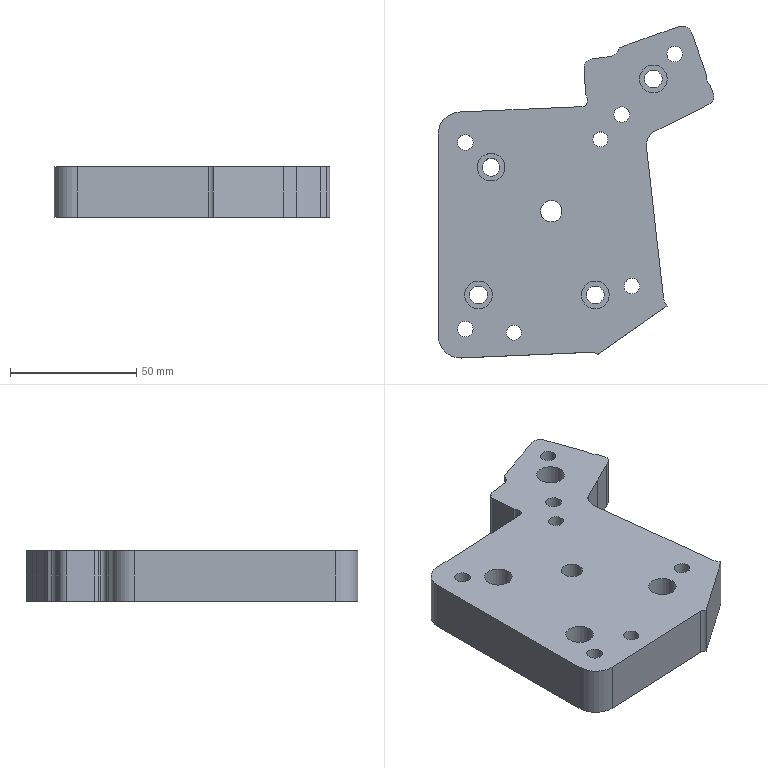Part | NX | features 23 2 | 1 solid | 60 faces | box 109.34 x 131.613 x 20 mm | volume 179684 mm3 | plane 31 | cylinder 29 | commonest cylinder face diameters 4.4 x5 6.2 x5 7 x4 11 x4 6.001 x2 12.4 x2